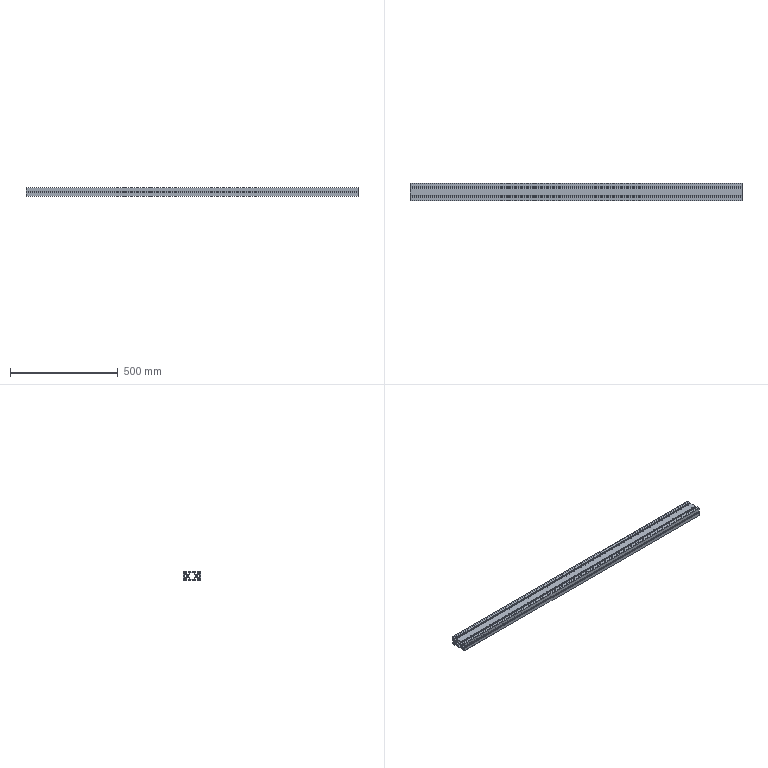Part | SolidWorks | features BaseBody 1 | 1 solid | 90 faces | box 1540 x 80 x 40 mm | volume 1897953 mm3 | plane 66 | cylinder 24 | commonest cylinder face diameters 10 x12 8 x8 6.2 x4